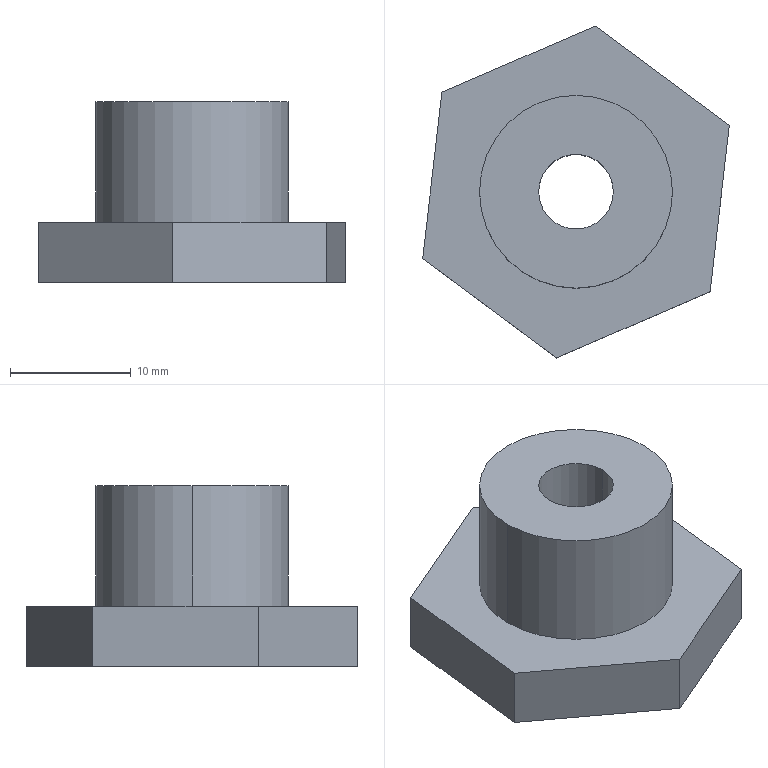Part | STEP file | Traction holder locating nut QY-1-40 | 1 solid | 13 faces | box 25.428 x 27.531 x 15 mm | volume 4052 mm3 | plane 9 | cylinder 4 | commonest cylinder face diameters 6.2 x2 16 x2
STEP:
#1=CARTESIAN_POINT('',(0.,0.,0.));
#2=DIRECTION('',(0.,0.,1.));
#3=DIRECTION('',(1.,0.,0.));
#4=AXIS2_PLACEMENT_3D('',#1,#2,#3);
#5=CARTESIAN_POINT('',(-3.1,0.,15.));
#6=VERTEX_POINT('',#5);
#7=CARTESIAN_POINT('',(-3.1,0.,0.));
#8=VERTEX_POINT('',#7);
#9=CARTESIAN_POINT('',(-3.1,0.,39.));
#10=DIRECTION('',(0.,0.,-1.));
#11=VECTOR('',#10,1.);
#12=LINE('',#9,#11);
#13=CARTESIAN_POINT('',(0.,0.,39.));
#14=DIRECTION('',(0.,0.,-1.));
#15=DIRECTION('',(-1.,0.,0.));
#16=AXIS2_PLACEMENT_3D('',#13,#14,#15);
#17=CYLINDRICAL_SURFACE('',#16,3.1);
#18=CARTESIAN_POINT('',(6.283,0.));
#19=DIRECTION('',(0.,1.));
#20=VECTOR('',#19,1.);
#21=LINE('',#18,#20);
#22=(GEOMETRIC_REPRESENTATION_CONTEXT(2)PARAMETRIC_REPRESENTATION_CONTEXT()REPRESENTATION_CONTEXT('',''));
#23=DEFINITIONAL_REPRESENTATION('',(#21),#22);
#24=PCURVE('',#17,#23);
#25=CARTESIAN_POINT('',(0.,0.,39.));
#26=DIRECTION('',(0.,0.,-1.));
#27=DIRECTION('',(-1.,0.,0.));
#28=AXIS2_PLACEMENT_3D('',#25,#26,#27);
#29=CYLINDRICAL_SURFACE('',#28,3.1);
#30=CARTESIAN_POINT('',(0.,0.));
#31=DIRECTION('',(0.,1.));
#32=VECTOR('',#31,1.);
#33=LINE('',#30,#32);
#34=(GEOMETRIC_REPRESENTATION_CONTEXT(2)PARAMETRIC_REPRESENTATION_CONTEXT()REPRESENTATION_CONTEXT('',''));
#35=DEFINITIONAL_REPRESENTATION('',(#33),#34);
#36=PCURVE('',#29,#35);
#37=SURFACE_CURVE('',#12,(#24,#36),.PCURVE_S1.);
#38=EDGE_CURVE('',#6,#8,#37,.T.);
#39=ORIENTED_EDGE('',*,*,#38,.T.);
#40=CARTESIAN_POINT('',(3.1,0.,0.));
#41=VERTEX_POINT('',#40);
#42=CARTESIAN_POINT('',(0.,0.,0.));
#43=DIRECTION('',(0.,0.,-1.));
#44=DIRECTION('',(-1.,0.,0.));
#45=AXIS2_PLACEMENT_3D('',#42,#43,#44);
#46=CIRCLE('',#45,3.1);
#47=CARTESIAN_POINT('',(0.,39.));
#48=DIRECTION('',(1.,0.));
#49=VECTOR('',#48,1.);
#50=LINE('',#47,#49);
#51=(GEOMETRIC_REPRESENTATION_CONTEXT(2)PARAMETRIC_REPRESENTATION_CONTEXT()REPRESENTATION_CONTEXT('',''));
#52=DEFINITIONAL_REPRESENTATION('',(#50),#51);
#53=PCURVE('',#17,#52);
#54=CARTESIAN_POINT('',(0.,0.,0.));
#55=DIRECTION('',(0.,0.,1.));
#56=DIRECTION('',(1.,0.,0.));
#57=AXIS2_PLACEMENT_3D('',#54,#55,#56);
#58=PLANE('',#57);
#59=CARTESIAN_POINT('',(-3.1,0.));
#60=CARTESIAN_POINT('',(-3.1,5.369));
#61=CARTESIAN_POINT('',(1.55,2.685));
#62=CARTESIAN_POINT('',(6.2,0.));
#63=CARTESIAN_POINT('',(1.55,-2.685));
#64=CARTESIAN_POINT('',(-3.1,-5.369));
#65=CARTESIAN_POINT('',(-3.1,0.));
#66=(BOUNDED_CURVE()B_SPLINE_CURVE(2,(#59,#60,#61,#62,#63,#64,#65),.UNSPECIFIED.,.T.,.F.)B_SPLINE_CURVE_WITH_KNOTS((1,2,2,2,2,1),(-2.094,0.,2.094,4.189,6.283,8.378),.UNSPECIFIED.)CURVE()GEOMETRIC_REPRESENTATION_ITEM()RATIONAL_B_SPLINE_CURVE((1.,0.5,1.,0.5,1.,0.5,1.))REPRESENTATION_ITEM(''));
#67=(GEOMETRIC_REPRESENTATION_CONTEXT(2)PARAMETRIC_REPRESENTATION_CONTEXT()REPRESENTATION_CONTEXT('',''));
#68=DEFINITIONAL_REPRESENTATION('',(#66),#67);
#69=PCURVE('',#58,#68);
#70=SURFACE_CURVE('',#46,(#53,#69),.PCURVE_S1.);
#71=EDGE_CURVE('',#41,#8,#70,.T.);
#72=ORIENTED_EDGE('',*,*,#71,.F.);
#73=CARTESIAN_POINT('',(3.1,0.,15.));
#74=VERTEX_POINT('',#73);
#75=CARTESIAN_POINT('',(3.1,0.,39.));
#76=DIRECTION('',(0.,0.,-1.));
#77=VECTOR('',#76,1.);
#78=LINE('',#75,#77);
#79=CARTESIAN_POINT('',(3.142,0.));
#80=DIRECTION('',(0.,1.));
#81=VECTOR('',#80,1.);
#82=LINE('',#79,#81);
#83=(GEOMETRIC_REPRESENTATION_CONTEXT(2)PARAMETRIC_REPRESENTATION_CONTEXT()REPRESENTATION_CONTEXT('',''));
#84=DEFINITIONAL_REPRESENTATION('',(#82),#83);
#85=PCURVE('',#17,#84);
#86=CARTESIAN_POINT('',(3.142,0.));
#87=DIRECTION('',(0.,1.));
#88=VECTOR('',#87,1.);
#89=LINE('',#86,#88);
#90=(GEOMETRIC_REPRESENTATION_CONTEXT(2)PARAMETRIC_REPRESENTATION_CONTEXT()REPRESENTATION_CONTEXT('',''));
#91=DEFINITIONAL_REPRESENTATION('',(#89),#90);
#92=PCURVE('',#29,#91);
#93=SURFACE_CURVE('',#78,(#85,#92),.PCURVE_S1.);
#94=EDGE_CURVE('',#74,#41,#93,.T.);
#95=ORIENTED_EDGE('',*,*,#94,.F.);
#96=CARTESIAN_POINT('',(0.,0.,15.));
#97=DIRECTION('',(0.,0.,1.));
#98=DIRECTION('',(1.,0.,0.));
#99=AXIS2_PLACEMENT_3D('',#96,#97,#98);
#100=CIRCLE('',#99,3.1);
#101=CARTESIAN_POINT('',(9.425,24.));
#102=DIRECTION('',(-1.,0.));
#103=VECTOR('',#102,1.);
#104=LINE('',#101,#103);
#105=(GEOMETRIC_REPRESENTATION_CONTEXT(2)PARAMETRIC_REPRESENTATION_CONTEXT()REPRESENTATION_CONTEXT('',''));
#106=DEFINITIONAL_REPRESENTATION('',(#104),#105);
#107=PCURVE('',#17,#106);
#108=CARTESIAN_POINT('',(0.,0.,15.));
#109=DIRECTION('',(0.,0.,1.));
#110=DIRECTION('',(1.,0.,0.));
#111=AXIS2_PLACEMENT_3D('',#108,#109,#110);
#112=PLANE('',#111);
#113=CARTESIAN_POINT('',(0.,0.));
#114=DIRECTION('',(1.,0.));
#115=AXIS2_PLACEMENT_2D('',#113,#114);
#116=CIRCLE('',#115,3.1);
#117=(GEOMETRIC_REPRESENTATION_CONTEXT(2)PARAMETRIC_REPRESENTATION_CONTEXT()REPRESENTATION_CONTEXT('',''));
#118=DEFINITIONAL_REPRESENTATION('',(#116),#117);
#119=PCURVE('',#112,#118);
#120=SURFACE_CURVE('',#100,(#107,#119),.PCURVE_S1.);
#121=EDGE_CURVE('',#6,#74,#120,.T.);
#122=ORIENTED_EDGE('',*,*,#121,.F.);
#123=EDGE_LOOP('',(#39,#72,#95,#122));
#124=FACE_BOUND('',#123,.F.);
#125=ADVANCED_FACE('',(#124),#17,.F.);
#126=CARTESIAN_POINT('',(8.,0.,15.));
#127=VERTEX_POINT('',#126);
#128=CARTESIAN_POINT('',(-8.,0.,15.));
#129=VERTEX_POINT('',#128);
#130=CARTESIAN_POINT('',(0.,0.,15.));
#131=DIRECTION('',(0.,0.,1.));
#132=DIRECTION('',(1.,0.,0.));
#133=AXIS2_PLACEMENT_3D('',#130,#131,#132);
#134=CIRCLE('',#133,8.);
#135=CARTESIAN_POINT('',(0.,0.,15.));
#136=DIRECTION('',(0.,0.,-1.));
#137=DIRECTION('',(-1.,0.,0.));
#138=AXIS2_PLACEMENT_3D('',#135,#136,#137);
#139=CYLINDRICAL_SURFACE('',#138,8.);
#140=CARTESIAN_POINT('',(3.142,0.));
#141=DIRECTION('',(-1.,0.));
#142=VECTOR('',#141,1.);
#143=LINE('',#140,#142);
#144=(GEOMETRIC_REPRESENTATION_CONTEXT(2)PARAMETRIC_REPRESENTATION_CONTEXT()REPRESENTATION_CONTEXT('',''));
#145=DEFINITIONAL_REPRESENTATION('',(#143),#144);
#146=PCURVE('',#139,#145);
#147=CARTESIAN_POINT('',(0.,0.));
#148=DIRECTION('',(1.,0.));
#149=AXIS2_PLACEMENT_2D('',#147,#148);
#150=CIRCLE('',#149,8.);
#151=(GEOMETRIC_REPRESENTATION_CONTEXT(2)PARAMETRIC_REPRESENTATION_CONTEXT()REPRESENTATION_CONTEXT('',''));
#152=DEFINITIONAL_REPRESENTATION('',(#150),#151);
#153=PCURVE('',#112,#152);
#154=SURFACE_CURVE('',#134,(#146,#153),.PCURVE_S1.);
#155=EDGE_CURVE('',#127,#129,#154,.T.);
#156=ORIENTED_EDGE('',*,*,#155,.F.);
#157=CARTESIAN_POINT('',(8.,0.,5.));
#158=VERTEX_POINT('',#157);
#159=CARTESIAN_POINT('',(8.,0.,15.));
#160=DIRECTION('',(0.,0.,-1.));
#161=VECTOR('',#160,1.);
#162=LINE('',#159,#161);
#163=CARTESIAN_POINT('',(3.142,0.));
#164=DIRECTION('',(0.,1.));
#165=VECTOR('',#164,1.);
#166=LINE('',#163,#165);
#167=(GEOMETRIC_REPRESENTATION_CONTEXT(2)PARAMETRIC_REPRESENTATION_CONTEXT()REPRESENTATION_CONTEXT('',''));
#168=DEFINITIONAL_REPRESENTATION('',(#166),#167);
#169=PCURVE('',#139,#168);
#170=CARTESIAN_POINT('',(0.,0.,15.));
#171=DIRECTION('',(0.,0.,-1.));
#172=DIRECTION('',(-1.,0.,0.));
#173=AXIS2_PLACEMENT_3D('',#170,#171,#172);
#174=CYLINDRICAL_SURFACE('',#173,8.);
#175=CARTESIAN_POINT('',(3.142,0.));
#176=DIRECTION('',(0.,1.));
#177=VECTOR('',#176,1.);
#178=LINE('',#175,#177);
#179=(GEOMETRIC_REPRESENTATION_CONTEXT(2)PARAMETRIC_REPRESENTATION_CONTEXT()REPRESENTATION_CONTEXT('',''));
#180=DEFINITIONAL_REPRESENTATION('',(#178),#179);
#181=PCURVE('',#174,#180);
#182=SURFACE_CURVE('',#162,(#169,#181),.PCURVE_S1.);
#183=EDGE_CURVE('',#127,#158,#182,.T.);
#184=ORIENTED_EDGE('',*,*,#183,.T.);
#185=CARTESIAN_POINT('',(-8.,0.,5.));
#186=VERTEX_POINT('',#185);
#187=CARTESIAN_POINT('',(0.,0.,5.));
#188=DIRECTION('',(0.,0.,-1.));
#189=DIRECTION('',(-1.,0.,0.));
#190=AXIS2_PLACEMENT_3D('',#187,#188,#189);
#191=CIRCLE('',#190,8.);
#192=CARTESIAN_POINT('',(0.,10.));
#193=DIRECTION('',(1.,0.));
#194=VECTOR('',#193,1.);
#195=LINE('',#192,#194);
#196=(GEOMETRIC_REPRESENTATION_CONTEXT(2)PARAMETRIC_REPRESENTATION_CONTEXT()REPRESENTATION_CONTEXT('',''));
#197=DEFINITIONAL_REPRESENTATION('',(#195),#196);
#198=PCURVE('',#139,#197);
#199=CARTESIAN_POINT('',(0.,0.,5.));
#200=DIRECTION('',(0.,0.,-1.));
#201=DIRECTION('',(-1.,0.,0.));
#202=AXIS2_PLACEMENT_3D('',#199,#200,#201);
#203=PLANE('',#202);
#204=CARTESIAN_POINT('',(0.,0.));
#205=DIRECTION('',(1.,0.));
#206=AXIS2_PLACEMENT_2D('',#204,#205);
#207=CIRCLE('',#206,8.);
#208=(GEOMETRIC_REPRESENTATION_CONTEXT(2)PARAMETRIC_REPRESENTATION_CONTEXT()REPRESENTATION_CONTEXT('',''));
#209=DEFINITIONAL_REPRESENTATION('',(#207),#208);
#210=PCURVE('',#203,#209);
#211=SURFACE_CURVE('',#191,(#198,#210),.PCURVE_S1.);
#212=EDGE_CURVE('',#186,#158,#211,.T.);
#213=ORIENTED_EDGE('',*,*,#212,.F.);
#214=CARTESIAN_POINT('',(-8.,0.,15.));
#215=DIRECTION('',(0.,0.,-1.));
#216=VECTOR('',#215,1.);
#217=LINE('',#214,#216);
#218=CARTESIAN_POINT('',(0.,0.));
#219=DIRECTION('',(0.,1.));
#220=VECTOR('',#219,1.);
#221=LINE('',#218,#220);
#222=(GEOMETRIC_REPRESENTATION_CONTEXT(2)PARAMETRIC_REPRESENTATION_CONTEXT()REPRESENTATION_CONTEXT('',''));
#223=DEFINITIONAL_REPRESENTATION('',(#221),#222);
#224=PCURVE('',#139,#223);
#225=CARTESIAN_POINT('',(6.283,0.));
#226=DIRECTION('',(0.,1.));
#227=VECTOR('',#226,1.);
#228=LINE('',#225,#227);
#229=(GEOMETRIC_REPRESENTATION_CONTEXT(2)PARAMETRIC_REPRESENTATION_CONTEXT()REPRESENTATION_CONTEXT('',''));
#230=DEFINITIONAL_REPRESENTATION('',(#228),#229);
#231=PCURVE('',#174,#230);
#232=SURFACE_CURVE('',#217,(#224,#231),.PCURVE_S1.);
#233=EDGE_CURVE('',#129,#186,#232,.T.);
#234=ORIENTED_EDGE('',*,*,#233,.F.);
#235=EDGE_LOOP('',(#156,#184,#213,#234));
#236=FACE_BOUND('',#235,.T.);
#237=ADVANCED_FACE('',(#236),#139,.T.);
#238=ORIENTED_EDGE('',*,*,#183,.F.);
#239=CARTESIAN_POINT('',(0.,0.,15.));
#240=DIRECTION('',(0.,0.,1.));
#241=DIRECTION('',(1.,0.,0.));
#242=AXIS2_PLACEMENT_3D('',#239,#240,#241);
#243=CIRCLE('',#242,8.);
#244=CARTESIAN_POINT('',(9.425,0.));
#245=DIRECTION('',(-1.,0.));
#246=VECTOR('',#245,1.);
#247=LINE('',#244,#246);
#248=(GEOMETRIC_REPRESENTATION_CONTEXT(2)PARAMETRIC_REPRESENTATION_CONTEXT()REPRESENTATION_CONTEXT('',''));
#249=DEFINITIONAL_REPRESENTATION('',(#247),#248);
#250=PCURVE('',#174,#249);
#251=CARTESIAN_POINT('',(0.,0.));
#252=DIRECTION('',(1.,0.));
#253=AXIS2_PLACEMENT_2D('',#251,#252);
#254=CIRCLE('',#253,8.);
#255=(GEOMETRIC_REPRESENTATION_CONTEXT(2)PARAMETRIC_REPRESENTATION_CONTEXT()REPRESENTATION_CONTEXT('',''));
#256=DEFINITIONAL_REPRESENTATION('',(#254),#255);
#257=PCURVE('',#112,#256);
#258=SURFACE_CURVE('',#243,(#250,#257),.PCURVE_S1.);
#259=EDGE_CURVE('',#129,#127,#258,.T.);
#260=ORIENTED_EDGE('',*,*,#259,.F.);
#261=ORIENTED_EDGE('',*,*,#233,.T.);
#262=CARTESIAN_POINT('',(0.,0.,5.));
#263=DIRECTION('',(0.,0.,-1.));
#264=DIRECTION('',(-1.,0.,0.));
#265=AXIS2_PLACEMENT_3D('',#262,#263,#264);
#266=CIRCLE('',#265,8.);
#267=CARTESIAN_POINT('',(0.,10.));
#268=DIRECTION('',(1.,0.));
#269=VECTOR('',#268,1.);
#270=LINE('',#267,#269);
#271=(GEOMETRIC_REPRESENTATION_CONTEXT(2)PARAMETRIC_REPRESENTATION_CONTEXT()REPRESENTATION_CONTEXT('',''));
#272=DEFINITIONAL_REPRESENTATION('',(#270),#271);
#273=PCURVE('',#174,#272);
#274=CARTESIAN_POINT('',(0.,0.));
#275=DIRECTION('',(1.,0.));
#276=AXIS2_PLACEMENT_2D('',#274,#275);
#277=CIRCLE('',#276,8.);
#278=(GEOMETRIC_REPRESENTATION_CONTEXT(2)PARAMETRIC_REPRESENTATION_CONTEXT()REPRESENTATION_CONTEXT('',''));
#279=DEFINITIONAL_REPRESENTATION('',(#277),#278);
#280=PCURVE('',#203,#279);
#281=SURFACE_CURVE('',#266,(#273,#280),.PCURVE_S1.);
#282=EDGE_CURVE('',#158,#186,#281,.T.);
#283=ORIENTED_EDGE('',*,*,#282,.F.);
#284=EDGE_LOOP('',(#238,#260,#261,#283));
#285=FACE_BOUND('',#284,.T.);
#286=ADVANCED_FACE('',(#285),#174,.T.);
#287=ORIENTED_EDGE('',*,*,#121,.F.);
#288=CARTESIAN_POINT('',(0.,0.,15.));
#289=DIRECTION('',(0.,0.,1.));
#290=DIRECTION('',(1.,0.,0.));
#291=AXIS2_PLACEMENT_3D('',#288,#289,#290);
#292=CIRCLE('',#291,3.1);
#293=CARTESIAN_POINT('',(0.,0.));
#294=DIRECTION('',(1.,0.));
#295=AXIS2_PLACEMENT_2D('',#293,#294);
#296=CIRCLE('',#295,3.1);
#297=(GEOMETRIC_REPRESENTATION_CONTEXT(2)PARAMETRIC_REPRESENTATION_CONTEXT()REPRESENTATION_CONTEXT('',''));
#298=DEFINITIONAL_REPRESENTATION('',(#296),#297);
#299=PCURVE('',#112,#298);
#300=CARTESIAN_POINT('',(3.142,24.));
#301=DIRECTION('',(-1.,0.));
#302=VECTOR('',#301,1.);
#303=LINE('',#300,#302);
#304=(GEOMETRIC_REPRESENTATION_CONTEXT(2)PARAMETRIC_REPRESENTATION_CONTEXT()REPRESENTATION_CONTEXT('',''));
#305=DEFINITIONAL_REPRESENTATION('',(#303),#304);
#306=PCURVE('',#29,#305);
#307=SURFACE_CURVE('',#292,(#299,#306),.PCURVE_S1.);
#308=EDGE_CURVE('',#74,#6,#307,.T.);
#309=ORIENTED_EDGE('',*,*,#308,.F.);
#310=EDGE_LOOP('',(#287,#309));
#311=FACE_BOUND('',#310,.T.);
#312=ORIENTED_EDGE('',*,*,#259,.T.);
#313=ORIENTED_EDGE('',*,*,#155,.T.);
#314=EDGE_LOOP('',(#312,#313));
#315=FACE_BOUND('',#314,.T.);
#316=ADVANCED_FACE('',(#311,#315),#112,.T.);
#317=CARTESIAN_POINT('',(-12.714,-5.509,0.));
#318=VERTEX_POINT('',#317);
#319=CARTESIAN_POINT('',(-11.128,8.256,0.));
#320=VERTEX_POINT('',#319);
#321=CARTESIAN_POINT('',(-12.714,-5.509,0.));
#322=DIRECTION('',(0.1145,0.9934,0.));
#323=VECTOR('',#322,1.);
#324=LINE('',#321,#323);
#325=CARTESIAN_POINT('',(-12.714,-5.509,5.));
#326=DIRECTION('',(-0.9934,0.1145,0.));
#327=DIRECTION('',(-0.1145,-0.9934,0.));
#328=AXIS2_PLACEMENT_3D('',#325,#326,#327);
#329=PLANE('',#328);
#330=CARTESIAN_POINT('',(0.,-5.));
#331=DIRECTION('',(-1.,0.));
#332=VECTOR('',#331,1.);
#333=LINE('',#330,#332);
#334=(GEOMETRIC_REPRESENTATION_CONTEXT(2)PARAMETRIC_REPRESENTATION_CONTEXT()REPRESENTATION_CONTEXT('',''));
#335=DEFINITIONAL_REPRESENTATION('',(#333),#334);
#336=PCURVE('',#329,#335);
#337=CARTESIAN_POINT('',(-12.714,-5.509));
#338=DIRECTION('',(0.1145,0.9934));
#339=VECTOR('',#338,1.);
#340=LINE('',#337,#339);
#341=(GEOMETRIC_REPRESENTATION_CONTEXT(2)PARAMETRIC_REPRESENTATION_CONTEXT()REPRESENTATION_CONTEXT('',''));
#342=DEFINITIONAL_REPRESENTATION('',(#340),#341);
#343=PCURVE('',#58,#342);
#344=SURFACE_CURVE('',#324,(#336,#343),.PCURVE_S1.);
#345=EDGE_CURVE('',#318,#320,#344,.T.);
#346=ORIENTED_EDGE('',*,*,#345,.F.);
#347=CARTESIAN_POINT('',(-12.714,-5.509,5.));
#348=VERTEX_POINT('',#347);
#349=CARTESIAN_POINT('',(-12.714,-5.509,5.));
#350=DIRECTION('',(0.,0.,-1.));
#351=VECTOR('',#350,1.);
#352=LINE('',#349,#351);
#353=CARTESIAN_POINT('',(0.,0.));
#354=DIRECTION('',(0.,-1.));
#355=VECTOR('',#354,1.);
#356=LINE('',#353,#355);
#357=(GEOMETRIC_REPRESENTATION_CONTEXT(2)PARAMETRIC_REPRESENTATION_CONTEXT()REPRESENTATION_CONTEXT('',''));
#358=DEFINITIONAL_REPRESENTATION('',(#356),#357);
#359=PCURVE('',#329,#358);
#360=CARTESIAN_POINT('',(-1.586,-13.765,5.));
#361=DIRECTION('',(-0.5958,-0.8031,0.));
#362=DIRECTION('',(0.8031,-0.5958,0.));
#363=AXIS2_PLACEMENT_3D('',#360,#361,#362);
#364=PLANE('',#363);
#365=CARTESIAN_POINT('',(-13.856,0.));
#366=DIRECTION('',(0.,-1.));
#367=VECTOR('',#366,1.);
#368=LINE('',#365,#367);
#369=(GEOMETRIC_REPRESENTATION_CONTEXT(2)PARAMETRIC_REPRESENTATION_CONTEXT()REPRESENTATION_CONTEXT('',''));
#370=DEFINITIONAL_REPRESENTATION('',(#368),#369);
#371=PCURVE('',#364,#370);
#372=SURFACE_CURVE('',#352,(#359,#371),.PCURVE_S1.);
#373=EDGE_CURVE('',#348,#318,#372,.T.);
#374=ORIENTED_EDGE('',*,*,#373,.F.);
#375=CARTESIAN_POINT('',(-11.128,8.256,5.));
#376=VERTEX_POINT('',#375);
#377=CARTESIAN_POINT('',(-12.714,-5.509,5.));
#378=DIRECTION('',(0.1145,0.9934,0.));
#379=VECTOR('',#378,1.);
#380=LINE('',#377,#379);
#381=CARTESIAN_POINT('',(0.,0.));
#382=DIRECTION('',(-1.,0.));
#383=VECTOR('',#382,1.);
#384=LINE('',#381,#383);
#385=(GEOMETRIC_REPRESENTATION_CONTEXT(2)PARAMETRIC_REPRESENTATION_CONTEXT()REPRESENTATION_CONTEXT('',''));
#386=DEFINITIONAL_REPRESENTATION('',(#384),#385);
#387=PCURVE('',#329,#386);
#388=CARTESIAN_POINT('',(12.714,-5.509));
#389=DIRECTION('',(-0.1145,0.9934));
#390=VECTOR('',#389,1.);
#391=LINE('',#388,#390);
#392=(GEOMETRIC_REPRESENTATION_CONTEXT(2)PARAMETRIC_REPRESENTATION_CONTEXT()REPRESENTATION_CONTEXT('',''));
#393=DEFINITIONAL_REPRESENTATION('',(#391),#392);
#394=PCURVE('',#203,#393);
#395=SURFACE_CURVE('',#380,(#387,#394),.PCURVE_S1.);
#396=EDGE_CURVE('',#348,#376,#395,.T.);
#397=ORIENTED_EDGE('',*,*,#396,.T.);
#398=CARTESIAN_POINT('',(-11.128,8.256,5.));
#399=DIRECTION('',(0.,0.,-1.));
#400=VECTOR('',#399,1.);
#401=LINE('',#398,#400);
#402=CARTESIAN_POINT('',(-13.856,0.));
#403=DIRECTION('',(0.,-1.));
#404=VECTOR('',#403,1.);
#405=LINE('',#402,#404);
#406=(GEOMETRIC_REPRESENTATION_CONTEXT(2)PARAMETRIC_REPRESENTATION_CONTEXT()REPRESENTATION_CONTEXT('',''));
#407=DEFINITIONAL_REPRESENTATION('',(#405),#406);
#408=PCURVE('',#329,#407);
#409=CARTESIAN_POINT('',(-11.128,8.256,5.));
#410=DIRECTION('',(-0.3976,0.9176,0.));
#411=DIRECTION('',(-0.9176,-0.3976,0.));
#412=AXIS2_PLACEMENT_3D('',#409,#410,#411);
#413=PLANE('',#412);
#414=CARTESIAN_POINT('',(0.,0.));
#415=DIRECTION('',(0.,-1.));
#416=VECTOR('',#415,1.);
#417=LINE('',#414,#416);
#418=(GEOMETRIC_REPRESENTATION_CONTEXT(2)PARAMETRIC_REPRESENTATION_CONTEXT()REPRESENTATION_CONTEXT('',''));
#419=DEFINITIONAL_REPRESENTATION('',(#417),#418);
#420=PCURVE('',#413,#419);
#421=SURFACE_CURVE('',#401,(#408,#420),.PCURVE_S1.);
#422=EDGE_CURVE('',#376,#320,#421,.T.);
#423=ORIENTED_EDGE('',*,*,#422,.T.);
#424=EDGE_LOOP('',(#346,#374,#397,#423));
#425=FACE_BOUND('',#424,.T.);
#426=ADVANCED_FACE('',(#425),#329,.T.);
#427=CARTESIAN_POINT('',(-1.586,-13.765,0.));
#428=VERTEX_POINT('',#427);
#429=CARTESIAN_POINT('',(-1.586,-13.765,0.));
#430=DIRECTION('',(-0.8031,0.5958,0.));
#431=VECTOR('',#430,1.);
#432=LINE('',#429,#431);
#433=CARTESIAN_POINT('',(0.,-5.));
#434=DIRECTION('',(-1.,0.));
#435=VECTOR('',#434,1.);
#436=LINE('',#433,#435);
#437=(GEOMETRIC_REPRESENTATION_CONTEXT(2)PARAMETRIC_REPRESENTATION_CONTEXT()REPRESENTATION_CONTEXT('',''));
#438=DEFINITIONAL_REPRESENTATION('',(#436),#437);
#439=PCURVE('',#364,#438);
#440=CARTESIAN_POINT('',(-1.586,-13.765));
#441=DIRECTION('',(-0.8031,0.5958));
#442=VECTOR('',#441,1.);
#443=LINE('',#440,#442);
#444=(GEOMETRIC_REPRESENTATION_CONTEXT(2)PARAMETRIC_REPRESENTATION_CONTEXT()REPRESENTATION_CONTEXT('',''));
#445=DEFINITIONAL_REPRESENTATION('',(#443),#444);
#446=PCURVE('',#58,#445);
#447=SURFACE_CURVE('',#432,(#439,#446),.PCURVE_S1.);
#448=EDGE_CURVE('',#428,#318,#447,.T.);
#449=ORIENTED_EDGE('',*,*,#448,.F.);
#450=CARTESIAN_POINT('',(-1.586,-13.765,5.));
#451=VERTEX_POINT('',#450);
#452=CARTESIAN_POINT('',(-1.586,-13.765,5.));
#453=DIRECTION('',(0.,0.,-1.));
#454=VECTOR('',#453,1.);
#455=LINE('',#452,#454);
#456=CARTESIAN_POINT('',(0.,0.));
#457=DIRECTION('',(0.,-1.));
#458=VECTOR('',#457,1.);
#459=LINE('',#456,#458);
#460=(GEOMETRIC_REPRESENTATION_CONTEXT(2)PARAMETRIC_REPRESENTATION_CONTEXT()REPRESENTATION_CONTEXT('',''));
#461=DEFINITIONAL_REPRESENTATION('',(#459),#460);
#462=PCURVE('',#364,#461);
#463=CARTESIAN_POINT('',(11.128,-8.256,5.));
#464=DIRECTION('',(0.3976,-0.9176,0.));
#465=DIRECTION('',(0.9176,0.3976,0.));
#466=AXIS2_PLACEMENT_3D('',#463,#464,#465);
#467=PLANE('',#466);
#468=CARTESIAN_POINT('',(-13.856,0.));
#469=DIRECTION('',(0.,-1.));
#470=VECTOR('',#469,1.);
#471=LINE('',#468,#470);
#472=(GEOMETRIC_REPRESENTATION_CONTEXT(2)PARAMETRIC_REPRESENTATION_CONTEXT()REPRESENTATION_CONTEXT('',''));
#473=DEFINITIONAL_REPRESENTATION('',(#471),#472);
#474=PCURVE('',#467,#473);
#475=SURFACE_CURVE('',#455,(#462,#474),.PCURVE_S1.);
#476=EDGE_CURVE('',#451,#428,#475,.T.);
#477=ORIENTED_EDGE('',*,*,#476,.F.);
#478=CARTESIAN_POINT('',(-1.586,-13.765,5.));
#479=DIRECTION('',(-0.8031,0.5958,0.));
#480=VECTOR('',#479,1.);
#481=LINE('',#478,#480);
#482=CARTESIAN_POINT('',(0.,0.));
#483=DIRECTION('',(-1.,0.));
#484=VECTOR('',#483,1.);
#485=LINE('',#482,#484);
#486=(GEOMETRIC_REPRESENTATION_CONTEXT(2)PARAMETRIC_REPRESENTATION_CONTEXT()REPRESENTATION_CONTEXT('',''));
#487=DEFINITIONAL_REPRESENTATION('',(#485),#486);
#488=PCURVE('',#364,#487);
#489=CARTESIAN_POINT('',(1.586,-13.765));
#490=DIRECTION('',(0.8031,0.5958));
#491=VECTOR('',#490,1.);
#492=LINE('',#489,#491);
#493=(GEOMETRIC_REPRESENTATION_CONTEXT(2)PARAMETRIC_REPRESENTATION_CONTEXT()REPRESENTATION_CONTEXT('',''));
#494=DEFINITIONAL_REPRESENTATION('',(#492),#493);
#495=PCURVE('',#203,#494);
#496=SURFACE_CURVE('',#481,(#488,#495),.PCURVE_S1.);
#497=EDGE_CURVE('',#451,#348,#496,.T.);
#498=ORIENTED_EDGE('',*,*,#497,.T.);
#499=ORIENTED_EDGE('',*,*,#373,.T.);
#500=EDGE_LOOP('',(#449,#477,#498,#499));
#501=FACE_BOUND('',#500,.T.);
#502=ADVANCED_FACE('',(#501),#364,.T.);
#503=CARTESIAN_POINT('',(11.128,-8.256,0.));
#504=VERTEX_POINT('',#503);
#505=CARTESIAN_POINT('',(11.128,-8.256,0.));
#506=DIRECTION('',(-0.9176,-0.3976,0.));
#507=VECTOR('',#506,1.);
#508=LINE('',#505,#507);
#509=CARTESIAN_POINT('',(0.,-5.));
#510=DIRECTION('',(-1.,0.));
#511=VECTOR('',#510,1.);
#512=LINE('',#509,#511);
#513=(GEOMETRIC_REPRESENTATION_CONTEXT(2)PARAMETRIC_REPRESENTATION_CONTEXT()REPRESENTATION_CONTEXT('',''));
#514=DEFINITIONAL_REPRESENTATION('',(#512),#513);
#515=PCURVE('',#467,#514);
#516=CARTESIAN_POINT('',(11.128,-8.256));
#517=DIRECTION('',(-0.9176,-0.3976));
#518=VECTOR('',#517,1.);
#519=LINE('',#516,#518);
#520=(GEOMETRIC_REPRESENTATION_CONTEXT(2)PARAMETRIC_REPRESENTATION_CONTEXT()REPRESENTATION_CONTEXT('',''));
#521=DEFINITIONAL_REPRESENTATION('',(#519),#520);
#522=PCURVE('',#58,#521);
#523=SURFACE_CURVE('',#508,(#515,#522),.PCURVE_S1.);
#524=EDGE_CURVE('',#504,#428,#523,.T.);
#525=ORIENTED_EDGE('',*,*,#524,.F.);
#526=CARTESIAN_POINT('',(11.128,-8.256,5.));
#527=VERTEX_POINT('',#526);
#528=CARTESIAN_POINT('',(11.128,-8.256,5.));
#529=DIRECTION('',(0.,0.,-1.));
#530=VECTOR('',#529,1.);
#531=LINE('',#528,#530);
#532=CARTESIAN_POINT('',(0.,0.));
#533=DIRECTION('',(0.,-1.));
#534=VECTOR('',#533,1.);
#535=LINE('',#532,#534);
#536=(GEOMETRIC_REPRESENTATION_CONTEXT(2)PARAMETRIC_REPRESENTATION_CONTEXT()REPRESENTATION_CONTEXT('',''));
#537=DEFINITIONAL_REPRESENTATION('',(#535),#536);
#538=PCURVE('',#467,#537);
#539=CARTESIAN_POINT('',(12.714,5.509,5.));
#540=DIRECTION('',(0.9934,-0.1145,0.));
#541=DIRECTION('',(0.1145,0.9934,0.));
#542=AXIS2_PLACEMENT_3D('',#539,#540,#541);
#543=PLANE('',#542);
#544=CARTESIAN_POINT('',(-13.856,0.));
#545=DIRECTION('',(0.,-1.));
#546=VECTOR('',#545,1.);
#547=LINE('',#544,#546);
#548=(GEOMETRIC_REPRESENTATION_CONTEXT(2)PARAMETRIC_REPRESENTATION_CONTEXT()REPRESENTATION_CONTEXT('',''));
#549=DEFINITIONAL_REPRESENTATION('',(#547),#548);
#550=PCURVE('',#543,#549);
#551=SURFACE_CURVE('',#531,(#538,#550),.PCURVE_S1.);
#552=EDGE_CURVE('',#527,#504,#551,.T.);
#553=ORIENTED_EDGE('',*,*,#552,.F.);
#554=CARTESIAN_POINT('',(11.128,-8.256,5.));
#555=DIRECTION('',(-0.9176,-0.3976,0.));
#556=VECTOR('',#555,1.);
#557=LINE('',#554,#556);
#558=CARTESIAN_POINT('',(0.,0.));
#559=DIRECTION('',(-1.,0.));
#560=VECTOR('',#559,1.);
#561=LINE('',#558,#560);
#562=(GEOMETRIC_REPRESENTATION_CONTEXT(2)PARAMETRIC_REPRESENTATION_CONTEXT()REPRESENTATION_CONTEXT('',''));
#563=DEFINITIONAL_REPRESENTATION('',(#561),#562);
#564=PCURVE('',#467,#563);
#565=CARTESIAN_POINT('',(-11.128,-8.256));
#566=DIRECTION('',(0.9176,-0.3976));
#567=VECTOR('',#566,1.);
#568=LINE('',#565,#567);
#569=(GEOMETRIC_REPRESENTATION_CONTEXT(2)PARAMETRIC_REPRESENTATION_CONTEXT()REPRESENTATION_CONTEXT('',''));
#570=DEFINITIONAL_REPRESENTATION('',(#568),#569);
#571=PCURVE('',#203,#570);
#572=SURFACE_CURVE('',#557,(#564,#571),.PCURVE_S1.);
#573=EDGE_CURVE('',#527,#451,#572,.T.);
#574=ORIENTED_EDGE('',*,*,#573,.T.);
#575=ORIENTED_EDGE('',*,*,#476,.T.);
#576=EDGE_LOOP('',(#525,#553,#574,#575));
#577=FACE_BOUND('',#576,.T.);
#578=ADVANCED_FACE('',(#577),#467,.T.);
#579=CARTESIAN_POINT('',(12.714,5.509,0.));
#580=VERTEX_POINT('',#579);
#581=CARTESIAN_POINT('',(12.714,5.509,0.));
#582=DIRECTION('',(-0.1145,-0.9934,0.));
#583=VECTOR('',#582,1.);
#584=LINE('',#581,#583);
#585=CARTESIAN_POINT('',(0.,-5.));
#586=DIRECTION('',(-1.,0.));
#587=VECTOR('',#586,1.);
#588=LINE('',#585,#587);
#589=(GEOMETRIC_REPRESENTATION_CONTEXT(2)PARAMETRIC_REPRESENTATION_CONTEXT()REPRESENTATION_CONTEXT('',''));
#590=DEFINITIONAL_REPRESENTATION('',(#588),#589);
#591=PCURVE('',#543,#590);
#592=CARTESIAN_POINT('',(12.714,5.509));
#593=DIRECTION('',(-0.1145,-0.9934));
#594=VECTOR('',#593,1.);
#595=LINE('',#592,#594);
#596=(GEOMETRIC_REPRESENTATION_CONTEXT(2)PARAMETRIC_REPRESENTATION_CONTEXT()REPRESENTATION_CONTEXT('',''));
#597=DEFINITIONAL_REPRESENTATION('',(#595),#596);
#598=PCURVE('',#58,#597);
#599=SURFACE_CURVE('',#584,(#591,#598),.PCURVE_S1.);
#600=EDGE_CURVE('',#580,#504,#599,.T.);
#601=ORIENTED_EDGE('',*,*,#600,.F.);
#602=CARTESIAN_POINT('',(12.714,5.509,5.));
#603=VERTEX_POINT('',#602);
#604=CARTESIAN_POINT('',(12.714,5.509,5.));
#605=DIRECTION('',(0.,0.,-1.));
#606=VECTOR('',#605,1.);
#607=LINE('',#604,#606);
#608=CARTESIAN_POINT('',(0.,0.));
#609=DIRECTION('',(0.,-1.));
#610=VECTOR('',#609,1.);
#611=LINE('',#608,#610);
#612=(GEOMETRIC_REPRESENTATION_CONTEXT(2)PARAMETRIC_REPRESENTATION_CONTEXT()REPRESENTATION_CONTEXT('',''));
#613=DEFINITIONAL_REPRESENTATION('',(#611),#612);
#614=PCURVE('',#543,#613);
#615=CARTESIAN_POINT('',(1.586,13.765,5.));
#616=DIRECTION('',(0.5958,0.8031,0.));
#617=DIRECTION('',(-0.8031,0.5958,0.));
#618=AXIS2_PLACEMENT_3D('',#615,#616,#617);
#619=PLANE('',#618);
#620=CARTESIAN_POINT('',(-13.856,0.));
#621=DIRECTION('',(0.,-1.));
#622=VECTOR('',#621,1.);
#623=LINE('',#620,#622);
#624=(GEOMETRIC_REPRESENTATION_CONTEXT(2)PARAMETRIC_REPRESENTATION_CONTEXT()REPRESENTATION_CONTEXT('',''));
#625=DEFINITIONAL_REPRESENTATION('',(#623),#624);
#626=PCURVE('',#619,#625);
#627=SURFACE_CURVE('',#607,(#614,#626),.PCURVE_S1.);
#628=EDGE_CURVE('',#603,#580,#627,.T.);
#629=ORIENTED_EDGE('',*,*,#628,.F.);
#630=CARTESIAN_POINT('',(12.714,5.509,5.));
#631=DIRECTION('',(-0.1145,-0.9934,0.));
#632=VECTOR('',#631,1.);
#633=LINE('',#630,#632);
#634=CARTESIAN_POINT('',(0.,0.));
#635=DIRECTION('',(-1.,0.));
#636=VECTOR('',#635,1.);
#637=LINE('',#634,#636);
#638=(GEOMETRIC_REPRESENTATION_CONTEXT(2)PARAMETRIC_REPRESENTATION_CONTEXT()REPRESENTATION_CONTEXT('',''));
#639=DEFINITIONAL_REPRESENTATION('',(#637),#638);
#640=PCURVE('',#543,#639);
#641=CARTESIAN_POINT('',(-12.714,5.509));
#642=DIRECTION('',(0.1145,-0.9934));
#643=VECTOR('',#642,1.);
#644=LINE('',#641,#643);
#645=(GEOMETRIC_REPRESENTATION_CONTEXT(2)PARAMETRIC_REPRESENTATION_CONTEXT()REPRESENTATION_CONTEXT('',''));
#646=DEFINITIONAL_REPRESENTATION('',(#644),#645);
#647=PCURVE('',#203,#646);
#648=SURFACE_CURVE('',#633,(#640,#647),.PCURVE_S1.);
#649=EDGE_CURVE('',#603,#527,#648,.T.);
#650=ORIENTED_EDGE('',*,*,#649,.T.);
#651=ORIENTED_EDGE('',*,*,#552,.T.);
#652=EDGE_LOOP('',(#601,#629,#650,#651));
#653=FACE_BOUND('',#652,.T.);
#654=ADVANCED_FACE('',(#653),#543,.T.);
#655=CARTESIAN_POINT('',(1.586,13.765,0.));
#656=VERTEX_POINT('',#655);
#657=CARTESIAN_POINT('',(1.586,13.765,0.));
#658=DIRECTION('',(0.8031,-0.5958,0.));
#659=VECTOR('',#658,1.);
#660=LINE('',#657,#659);
#661=CARTESIAN_POINT('',(0.,-5.));
#662=DIRECTION('',(-1.,0.));
#663=VECTOR('',#662,1.);
#664=LINE('',#661,#663);
#665=(GEOMETRIC_REPRESENTATION_CONTEXT(2)PARAMETRIC_REPRESENTATION_CONTEXT()REPRESENTATION_CONTEXT('',''));
#666=DEFINITIONAL_REPRESENTATION('',(#664),#665);
#667=PCURVE('',#619,#666);
#668=CARTESIAN_POINT('',(1.586,13.765));
#669=DIRECTION('',(0.8031,-0.5958));
#670=VECTOR('',#669,1.);
#671=LINE('',#668,#670);
#672=(GEOMETRIC_REPRESENTATION_CONTEXT(2)PARAMETRIC_REPRESENTATION_CONTEXT()REPRESENTATION_CONTEXT('',''));
#673=DEFINITIONAL_REPRESENTATION('',(#671),#672);
#674=PCURVE('',#58,#673);
#675=SURFACE_CURVE('',#660,(#667,#674),.PCURVE_S1.);
#676=EDGE_CURVE('',#656,#580,#675,.T.);
#677=ORIENTED_EDGE('',*,*,#676,.F.);
#678=CARTESIAN_POINT('',(1.586,13.765,5.));
#679=VERTEX_POINT('',#678);
#680=CARTESIAN_POINT('',(1.586,13.765,5.));
#681=DIRECTION('',(0.,0.,-1.));
#682=VECTOR('',#681,1.);
#683=LINE('',#680,#682);
#684=CARTESIAN_POINT('',(0.,0.));
#685=DIRECTION('',(0.,-1.));
#686=VECTOR('',#685,1.);
#687=LINE('',#684,#686);
#688=(GEOMETRIC_REPRESENTATION_CONTEXT(2)PARAMETRIC_REPRESENTATION_CONTEXT()REPRESENTATION_CONTEXT('',''));
#689=DEFINITIONAL_REPRESENTATION('',(#687),#688);
#690=PCURVE('',#619,#689);
#691=CARTESIAN_POINT('',(-13.856,0.));
#692=DIRECTION('',(0.,-1.));
#693=VECTOR('',#692,1.);
#694=LINE('',#691,#693);
#695=(GEOMETRIC_REPRESENTATION_CONTEXT(2)PARAMETRIC_REPRESENTATION_CONTEXT()REPRESENTATION_CONTEXT('',''));
#696=DEFINITIONAL_REPRESENTATION('',(#694),#695);
#697=PCURVE('',#413,#696);
#698=SURFACE_CURVE('',#683,(#690,#697),.PCURVE_S1.);
#699=EDGE_CURVE('',#679,#656,#698,.T.);
#700=ORIENTED_EDGE('',*,*,#699,.F.);
#701=CARTESIAN_POINT('',(1.586,13.765,5.));
#702=DIRECTION('',(0.8031,-0.5958,0.));
#703=VECTOR('',#702,1.);
#704=LINE('',#701,#703);
#705=CARTESIAN_POINT('',(0.,0.));
#706=DIRECTION('',(-1.,0.));
#707=VECTOR('',#706,1.);
#708=LINE('',#705,#707);
#709=(GEOMETRIC_REPRESENTATION_CONTEXT(2)PARAMETRIC_REPRESENTATION_CONTEXT()REPRESENTATION_CONTEXT('',''));
#710=DEFINITIONAL_REPRESENTATION('',(#708),#709);
#711=PCURVE('',#619,#710);
#712=CARTESIAN_POINT('',(-1.586,13.765));
#713=DIRECTION('',(-0.8031,-0.5958));
#714=VECTOR('',#713,1.);
#715=LINE('',#712,#714);
#716=(GEOMETRIC_REPRESENTATION_CONTEXT(2)PARAMETRIC_REPRESENTATION_CONTEXT()REPRESENTATION_CONTEXT('',''));
#717=DEFINITIONAL_REPRESENTATION('',(#715),#716);
#718=PCURVE('',#203,#717);
#719=SURFACE_CURVE('',#704,(#711,#718),.PCURVE_S1.);
#720=EDGE_CURVE('',#679,#603,#719,.T.);
#721=ORIENTED_EDGE('',*,*,#720,.T.);
#722=ORIENTED_EDGE('',*,*,#628,.T.);
#723=EDGE_LOOP('',(#677,#700,#721,#722));
#724=FACE_BOUND('',#723,.T.);
#725=ADVANCED_FACE('',(#724),#619,.T.);
#726=CARTESIAN_POINT('',(-11.128,8.256,0.));
#727=DIRECTION('',(0.9176,0.3976,0.));
#728=VECTOR('',#727,1.);
#729=LINE('',#726,#728);
#730=CARTESIAN_POINT('',(0.,-5.));
#731=DIRECTION('',(-1.,0.));
#732=VECTOR('',#731,1.);
#733=LINE('',#730,#732);
#734=(GEOMETRIC_REPRESENTATION_CONTEXT(2)PARAMETRIC_REPRESENTATION_CONTEXT()REPRESENTATION_CONTEXT('',''));
#735=DEFINITIONAL_REPRESENTATION('',(#733),#734);
#736=PCURVE('',#413,#735);
#737=CARTESIAN_POINT('',(-11.128,8.256));
#738=DIRECTION('',(0.9176,0.3976));
#739=VECTOR('',#738,1.);
#740=LINE('',#737,#739);
#741=(GEOMETRIC_REPRESENTATION_CONTEXT(2)PARAMETRIC_REPRESENTATION_CONTEXT()REPRESENTATION_CONTEXT('',''));
#742=DEFINITIONAL_REPRESENTATION('',(#740),#741);
#743=PCURVE('',#58,#742);
#744=SURFACE_CURVE('',#729,(#736,#743),.PCURVE_S1.);
#745=EDGE_CURVE('',#320,#656,#744,.T.);
#746=ORIENTED_EDGE('',*,*,#745,.F.);
#747=ORIENTED_EDGE('',*,*,#422,.F.);
#748=CARTESIAN_POINT('',(-11.128,8.256,5.));
#749=DIRECTION('',(0.9176,0.3976,0.));
#750=VECTOR('',#749,1.);
#751=LINE('',#748,#750);
#752=CARTESIAN_POINT('',(0.,0.));
#753=DIRECTION('',(-1.,0.));
#754=VECTOR('',#753,1.);
#755=LINE('',#752,#754);
#756=(GEOMETRIC_REPRESENTATION_CONTEXT(2)PARAMETRIC_REPRESENTATION_CONTEXT()REPRESENTATION_CONTEXT('',''));
#757=DEFINITIONAL_REPRESENTATION('',(#755),#756);
#758=PCURVE('',#413,#757);
#759=CARTESIAN_POINT('',(11.128,8.256));
#760=DIRECTION('',(-0.9176,0.3976));
#761=VECTOR('',#760,1.);
#762=LINE('',#759,#761);
#763=(GEOMETRIC_REPRESENTATION_CONTEXT(2)PARAMETRIC_REPRESENTATION_CONTEXT()REPRESENTATION_CONTEXT('',''));
#764=DEFINITIONAL_REPRESENTATION('',(#762),#763);
#765=PCURVE('',#203,#764);
#766=SURFACE_CURVE('',#751,(#758,#765),.PCURVE_S1.);
#767=EDGE_CURVE('',#376,#679,#766,.T.);
#768=ORIENTED_EDGE('',*,*,#767,.T.);
#769=ORIENTED_EDGE('',*,*,#699,.T.);
#770=EDGE_LOOP('',(#746,#747,#768,#769));
#771=FACE_BOUND('',#770,.T.);
#772=ADVANCED_FACE('',(#771),#413,.T.);
#773=ORIENTED_EDGE('',*,*,#212,.T.);
#774=ORIENTED_EDGE('',*,*,#282,.T.);
#775=EDGE_LOOP('',(#773,#774));
#776=FACE_BOUND('',#775,.T.);
#777=ORIENTED_EDGE('',*,*,#396,.F.);
#778=ORIENTED_EDGE('',*,*,#497,.F.);
#779=ORIENTED_EDGE('',*,*,#573,.F.);
#780=ORIENTED_EDGE('',*,*,#649,.F.);
#781=ORIENTED_EDGE('',*,*,#720,.F.);
#782=ORIENTED_EDGE('',*,*,#767,.F.);
#783=EDGE_LOOP('',(#777,#778,#779,#780,#781,#782));
#784=FACE_BOUND('',#783,.T.);
#785=ADVANCED_FACE('',(#776,#784),#203,.F.);
#786=CARTESIAN_POINT('',(0.,0.,0.));
#787=DIRECTION('',(0.,0.,-1.));
#788=DIRECTION('',(-1.,0.,0.));
#789=AXIS2_PLACEMENT_3D('',#786,#787,#788);
#790=CIRCLE('',#789,3.1);
#791=CARTESIAN_POINT('',(-3.1,0.));
#792=CARTESIAN_POINT('',(-3.1,5.369));
#793=CARTESIAN_POINT('',(1.55,2.685));
#794=CARTESIAN_POINT('',(6.2,0.));
#795=CARTESIAN_POINT('',(1.55,-2.685));
#796=CARTESIAN_POINT('',(-3.1,-5.369));
#797=CARTESIAN_POINT('',(-3.1,0.));
#798=(BOUNDED_CURVE()B_SPLINE_CURVE(2,(#791,#792,#793,#794,#795,#796,#797),.UNSPECIFIED.,.T.,.F.)B_SPLINE_CURVE_WITH_KNOTS((1,2,2,2,2,1),(-2.094,0.,2.094,4.189,6.283,8.378),.UNSPECIFIED.)CURVE()GEOMETRIC_REPRESENTATION_ITEM()RATIONAL_B_SPLINE_CURVE((1.,0.5,1.,0.5,1.,0.5,1.))REPRESENTATION_ITEM(''));
#799=(GEOMETRIC_REPRESENTATION_CONTEXT(2)PARAMETRIC_REPRESENTATION_CONTEXT()REPRESENTATION_CONTEXT('',''));
#800=DEFINITIONAL_REPRESENTATION('',(#798),#799);
#801=PCURVE('',#58,#800);
#802=CARTESIAN_POINT('',(0.,39.));
#803=DIRECTION('',(1.,0.));
#804=VECTOR('',#803,1.);
#805=LINE('',#802,#804);
#806=(GEOMETRIC_REPRESENTATION_CONTEXT(2)PARAMETRIC_REPRESENTATION_CONTEXT()REPRESENTATION_CONTEXT('',''));
#807=DEFINITIONAL_REPRESENTATION('',(#805),#806);
#808=PCURVE('',#29,#807);
#809=SURFACE_CURVE('',#790,(#801,#808),.PCURVE_S1.);
#810=EDGE_CURVE('',#8,#41,#809,.T.);
#811=ORIENTED_EDGE('',*,*,#810,.F.);
#812=ORIENTED_EDGE('',*,*,#71,.F.);
#813=EDGE_LOOP('',(#811,#812));
#814=FACE_BOUND('',#813,.T.);
#815=ORIENTED_EDGE('',*,*,#345,.T.);
#816=ORIENTED_EDGE('',*,*,#745,.T.);
#817=ORIENTED_EDGE('',*,*,#676,.T.);
#818=ORIENTED_EDGE('',*,*,#600,.T.);
#819=ORIENTED_EDGE('',*,*,#524,.T.);
#820=ORIENTED_EDGE('',*,*,#448,.T.);
#821=EDGE_LOOP('',(#815,#816,#817,#818,#819,#820));
#822=FACE_BOUND('',#821,.T.);
#823=ADVANCED_FACE('',(#814,#822),#58,.F.);
#824=ORIENTED_EDGE('',*,*,#810,.F.);
#825=ORIENTED_EDGE('',*,*,#38,.F.);
#826=ORIENTED_EDGE('',*,*,#308,.F.);
#827=ORIENTED_EDGE('',*,*,#94,.T.);
#828=EDGE_LOOP('',(#824,#825,#826,#827));
#829=FACE_BOUND('',#828,.F.);
#830=ADVANCED_FACE('',(#829),#29,.F.);
#831=CLOSED_SHELL('',(#125,#237,#286,#316,#426,#502,#578,#654,#725,#772,#785,#823,#830));
#832=MANIFOLD_SOLID_BREP('',#831);
#833=(LENGTH_UNIT()NAMED_UNIT(*)SI_UNIT(.MILLI.,.METRE.));
#834=UNCERTAINTY_MEASURE_WITH_UNIT(LENGTH_MEASURE(0.0000001),#833,'','');
#835=(NAMED_UNIT(*)PLANE_ANGLE_UNIT()SI_UNIT($,.RADIAN.));
#836=(NAMED_UNIT(*)SI_UNIT($,.STERADIAN.)SOLID_ANGLE_UNIT());
#837=(GEOMETRIC_REPRESENTATION_CONTEXT(3)GLOBAL_UNCERTAINTY_ASSIGNED_CONTEXT((#834))GLOBAL_UNIT_ASSIGNED_CONTEXT((#833,#835,#836))REPRESENTATION_CONTEXT('',''));
#838=ADVANCED_BREP_SHAPE_REPRESENTATION('',(#4,#832),#837);